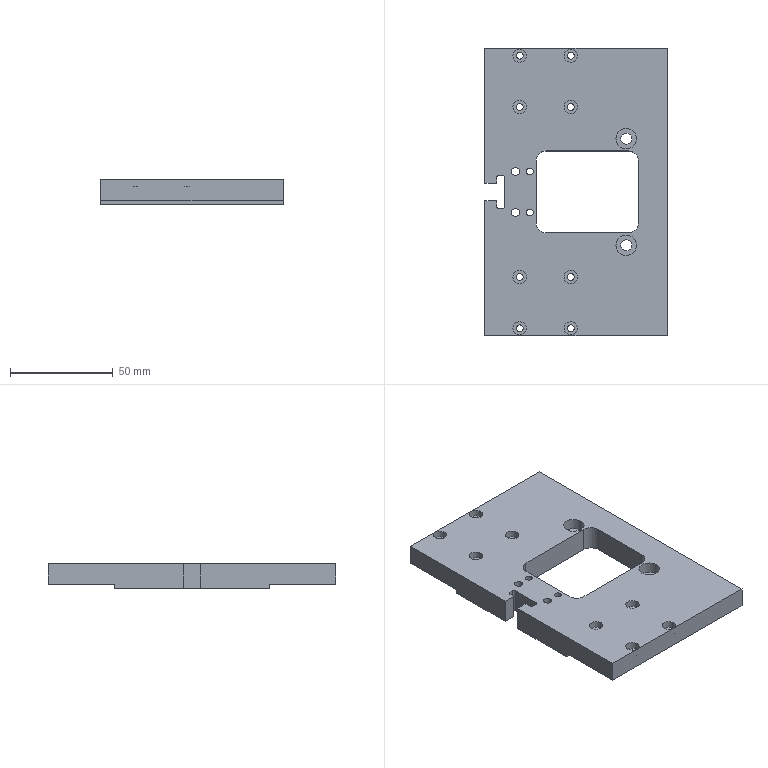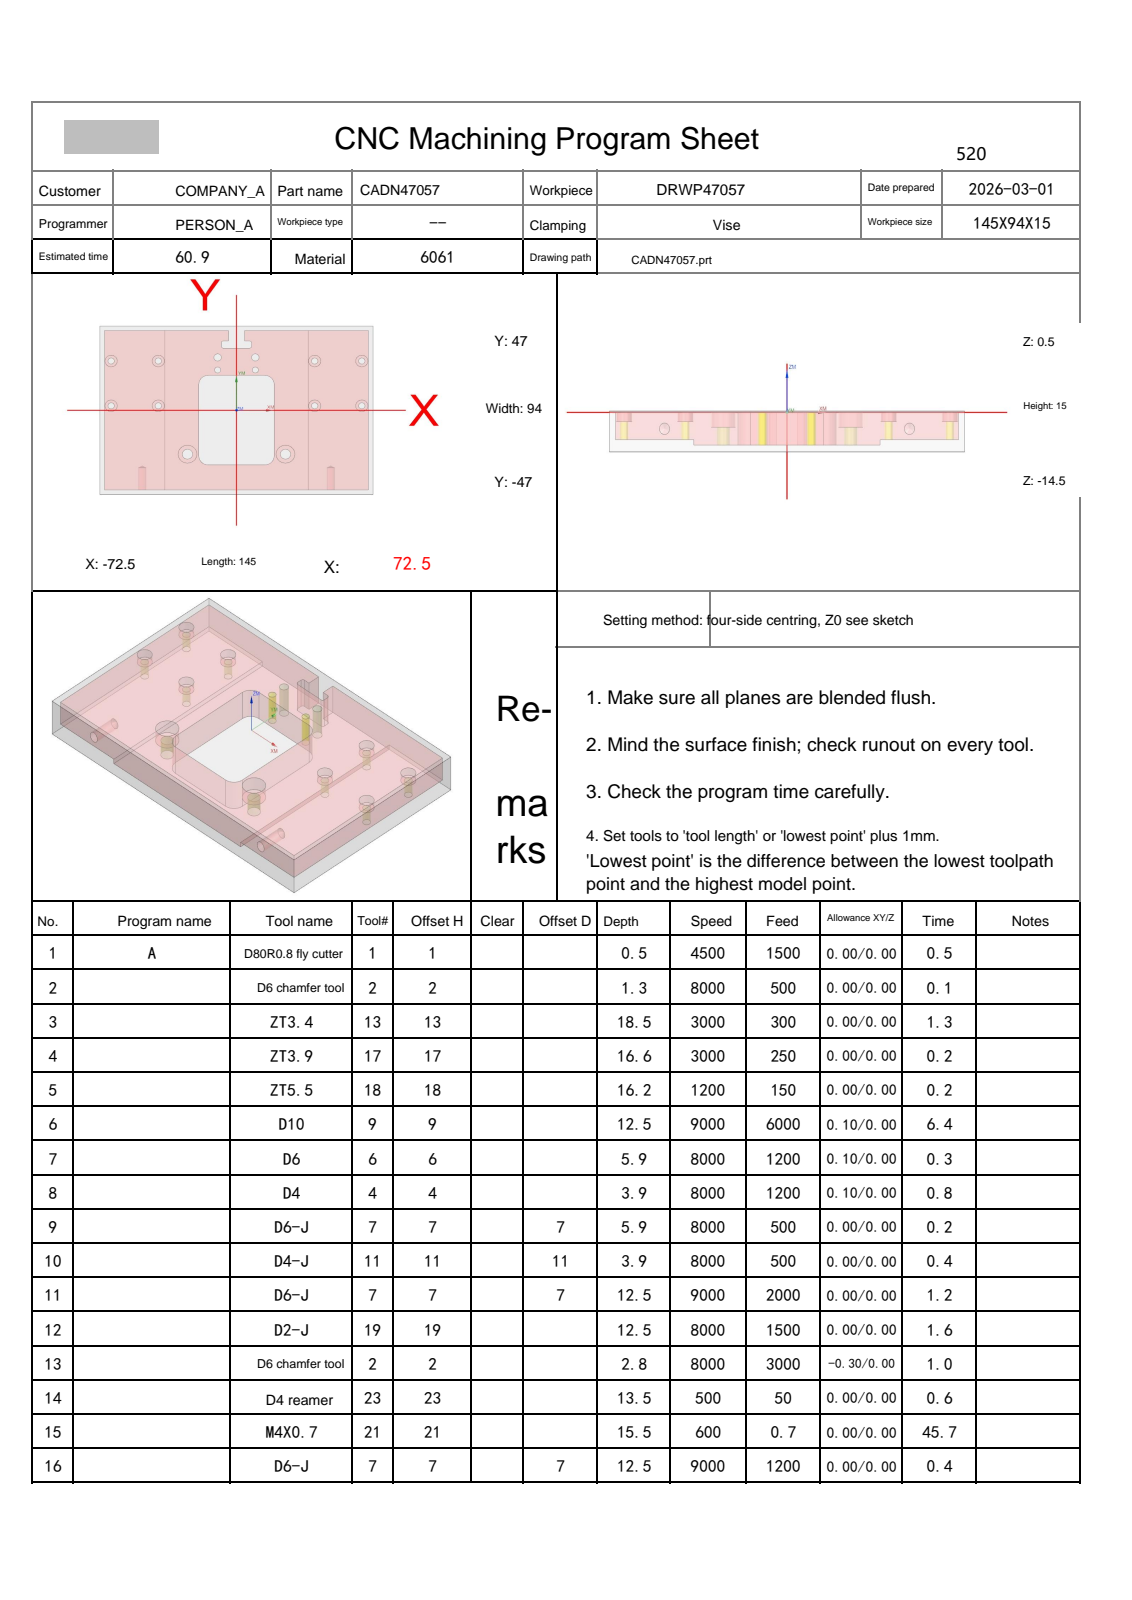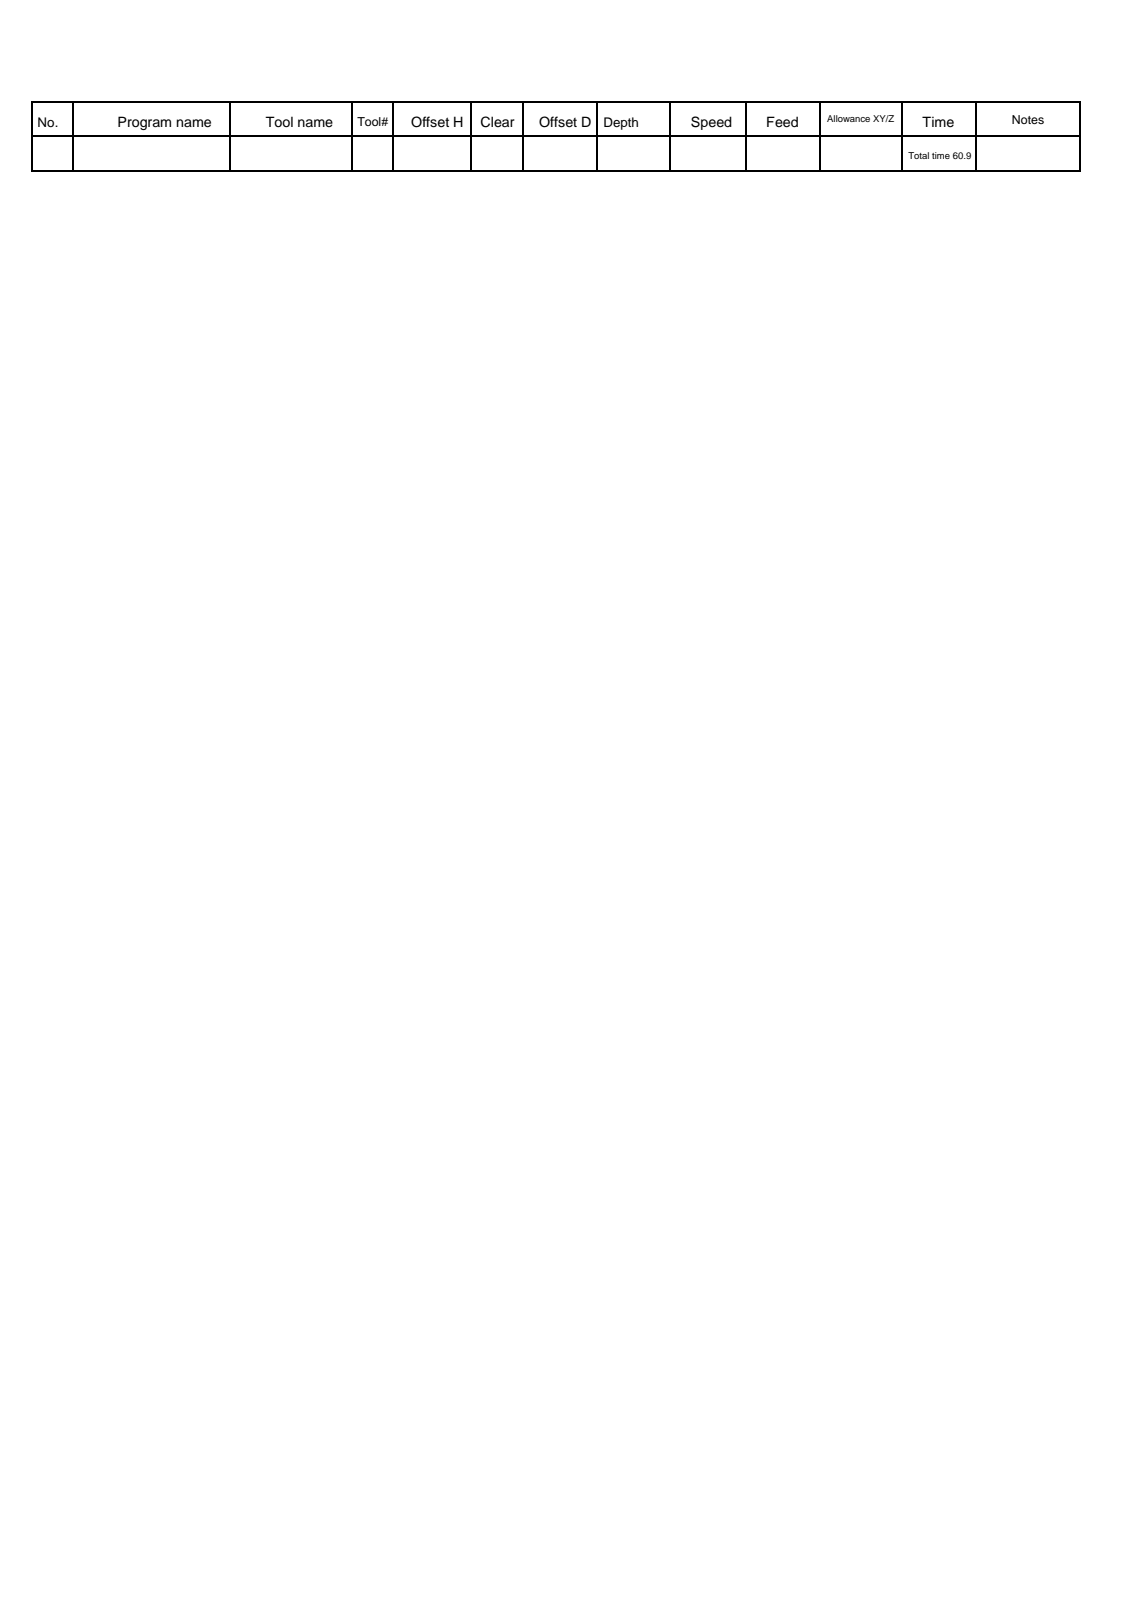NC program | NX | posted by the shop | part box 89 x 140 x 12 mm
Lines 1 to 948 of 6684:
%
O0001
(Machine time: 106.83 MIN)
(===Total Tool:13===)
(T1=D80R0.8 fly cutter D=80.  R=0.8  D-  H01 Z=0.    )
(T2=D6 chamfer tool   D=6.   R=0.   D-  H02 Z=-2.3  )
(T13=ZT3.4  D=3.4  DR_a=118 D-  H13 Z=-18.  )
(T17=ZT3.9  D=3.9  DR_a=120 D-  H17 Z=-16.13)
(T18=ZT5.5  D=5.5  DR_a=118 D-  H18 Z=-15.65)
(T9=D10     D=10.  R=0.   D-  H09 Z=-12.  )
(T6=D6      D=6.   R=0.   D-  H06 Z=-5.4  )
(T4=D4      D=4.   R=0.   D-  H04 Z=-3.4  )
(T7=D6-J    D=6.   R=0.   D7  H07 Z=-12.  )
(T11=D4-J   D=4.   R=0.   D11 H11 Z=-3.4  )
(T19=D2-J   D=2.   R=0.   D-  H19 Z=-12.  )
(T23=D4 reamer   D=4.   DR_a=180 D-  H23 Z=-13.  )
(T21=M4X0.7 D=3.3  DR_a=180 D-  H21 Z=-15.  )
G80 G90 G17 G49 G40
G91 G28 Z0
M01
N1 T01 M06
(D80R0.8 fly cutter  D=80. R=0.8 H=01 ce=0.00 di=0.00)
G00 G90 G54 X-115. Y42.25 M03 S4500
G43 H01 Z50.
M08
Z2.
G01 Z0.0 F1500.
X-110.
X110.
Y0.0
X-110.
Y-42.25
X110.
X115.
Z2.
G00 Z50.
G91 G28 Z0.0
M05
M09
G91 G28 Z0.0
M01
N2 T02 M06
(D6 chamfer tool  D=6. R=0. H=02 ce=0.00 di=0.00)
G00 G90 G54 X26. Y-24.5 M03 S8000
G43 H02 Z50.
M08
G98 G81 X26. Y-24.5 Z-.8 R1. F500.
X41.5 Y2.5
X66.5
Y27.5
X41.5
X10. Y29.5
Y22.5
X-10.
Y29.5
X-41.5 Y27.5
X-66.5
Y2.5
X-41.5
X-26. Y-24.5
G80
G00 Z50.
G91 G28 Z0.0
M05
M09
G91 G28 Z0.0
M01
N3 T13 M06
(ZT3.4 D=3.4 DR_a=118 H=13)
G00 G90 G54 X-10. Y22.5 M03 S3000
G43 H13 Z50.
M08
G98 G83 X-10. Y22.5 Z-18. R1. F300. Q2.
X10.
G80
G00 Z50.
G00 G90 X-66.5 Y2.5 M03 S2800
Z50.
G98 G83 X-66.5 Y2.5 Z-13.021 R1. F100. Q2.
Y27.5
X-41.5
Y2.5
X41.5
X66.5
Y27.5
X41.5
G80
G00 Z50.
G91 G28 Z0.0
M05
M09
G91 G28 Z0.0
M01
N4 T17 M06
(ZT3.9 D=3.9 DR_a=120 H=17)
G00 G90 G54 X-10. Y29.5 M03 S3000
G43 H17 Z50.
M08
G98 G83 X-10. Y29.5 Z-16.126 R1. F250. Q2.
X10.
G80
G00 Z50.
G91 G28 Z0.0
M05
M09
G91 G28 Z0.0
M01
N5 T18 M06
(ZT5.5 D=5.5 DR_a=118 H=18)
G00 G90 G54 X-26. Y-24.5 M03 S1200
G43 H18 Z50.
M08
G98 G83 X-26. Y-24.5 Z-15.652 R1. F150. Q2.
X26.
G80
G00 Z50.
G91 G28 Z0.0
M05
M09
G91 G28 Z0.0
M01
N6 T09 M06
(D10  D=10. R=0. H=09 ce=0.10 di=0.00)
G00 G90 G54 X14.9 Y-5.5 M03 S9000
G43 H09 Z50.
M08
Z.5
G01 Y14.4 Z.458 F1200.
X-14.9 Z.395
Y-25.4 Z.31
X14.9 Z.247
Y14.4 Z.163
X-14.9 Z.099
Y-25.4 Z.015
X14.9 Z-.048
Y14.4 Z-.133
X-14.9 Z-.196
Y-25.4 Z-.28
X14.9 Z-.344
Y14.4 Z-.428
X-14.9 Z-.491
Y-25.4 Z-.576
X14.9 Z-.639
Y14.4 Z-.723
X-14.9 Z-.786
Y-25.4 Z-.871
X14.9 Z-.934
Y14.4 Z-1.018
X-14.9 Z-1.082
Y-25.4 Z-1.166
X14.9 Z-1.229
Y14.4 Z-1.314
X-14.9 Z-1.377
Y-25.4 Z-1.461
X14.9 Z-1.524
Y14.4 Z-1.609
X-14.9 Z-1.672
Y-25.4 Z-1.756
X14.9 Z-1.82
Y14.4 Z-1.904
X-14.9 Z-1.967
Y-25.4 Z-2.052
X14.9 Z-2.115
Y14.4 Z-2.199
X-14.9 Z-2.263
Y-25.4 Z-2.347
X14.9 Z-2.41
Y14.4 Z-2.495
X-14.9 Z-2.558
Y-25.4 Z-2.642
X14.9 Z-2.705
Y14.4 Z-2.79
X-14.9 Z-2.853
Y-25.4 Z-2.937
X14.9 Z-3.001
Y14.4 Z-3.085
X-14.9 Z-3.148
Y-25.4 Z-3.233
X14.9 Z-3.296
Y14.4 Z-3.38
X-14.9 Z-3.444
Y-25.4 Z-3.528
X14.9 Z-3.591
Y14.4 Z-3.676
X-14.9 Z-3.739
Y-25.4 Z-3.823
X14.9 Z-3.886
Y14.4 Z-3.971
X-14.9 Z-4.034
Y-25.4 Z-4.118
X14.9 Z-4.182
Y14.4 Z-4.266
X-14.9 Z-4.329
Y-25.4 Z-4.414
X14.9 Z-4.477
Y14.4 Z-4.561
X-14.9 Z-4.624
Y-25.4 Z-4.709
X14.9 Z-4.772
Y14.4 Z-4.856
X-14.9 Z-4.92
Y-25.4 Z-5.004
X14.9 Z-5.067
Y14.4 Z-5.152
X-14.9 Z-5.215
Y-25.4 Z-5.299
X14.9 Z-5.363
Y14.4 Z-5.447
X-14.9 Z-5.51
Y-25.4 Z-5.595
X14.9 Z-5.658
Y14.4 Z-5.742
X-14.9 Z-5.805
Y-25.4 Z-5.89
X14.9 Z-5.953
Y14.4 Z-6.037
X-14.9 Z-6.101
Y-25.4 Z-6.185
X14.9 Z-6.248
Y14.4 Z-6.333
X-14.9 Z-6.396
Y-25.4 Z-6.48
X14.9 Z-6.544
Y14.4 Z-6.628
X-14.9 Z-6.691
Y-25.4 Z-6.776
X14.9 Z-6.839
Y14.4 Z-6.923
X-14.9 Z-6.986
Y-25.4 Z-7.071
X14.9 Z-7.134
Y14.4 Z-7.218
X-14.9 Z-7.282
Y-25.4 Z-7.366
X14.9 Z-7.429
Y14.4 Z-7.514
X-14.9 Z-7.577
Y-25.4 Z-7.661
X14.9 Z-7.724
Y14.4 Z-7.809
X-14.9 Z-7.872
Y-25.4 Z-7.956
X14.9 Z-8.02
Y14.4 Z-8.104
X-14.9 Z-8.167
Y-25.4 Z-8.252
X14.9 Z-8.315
Y14.4 Z-8.399
X-14.9 Z-8.463
Y-25.4 Z-8.547
X14.9 Z-8.61
Y14.4 Z-8.695
X-14.9 Z-8.758
Y-25.4 Z-8.842
X14.9 Z-8.905
Y14.4 Z-8.99
X-14.9 Z-9.053
Y-25.4 Z-9.137
X14.9 Z-9.201
Y14.4 Z-9.285
X-14.9 Z-9.348
Y-25.4 Z-9.433
X14.9 Z-9.496
Y14.4 Z-9.58
X-14.9 Z-9.644
Y-25.4 Z-9.728
X14.9 Z-9.791
Y14.4 Z-9.876
X-14.9 Z-9.939
Y-25.4 Z-10.023
X14.9 Z-10.086
Y14.4 Z-10.171
X-14.9 Z-10.234
Y-25.4 Z-10.318
X14.9 Z-10.382
Y14.4 Z-10.466
X-14.9 Z-10.529
Y-25.4 Z-10.614
X14.9 Z-10.677
Y14.4 Z-10.761
X-14.9 Z-10.824
Y-25.4 Z-10.909
X14.9 Z-10.972
Y14.4 Z-11.056
X-14.9 Z-11.12
Y-25.4 Z-11.204
X14.9 Z-11.267
Y14.4 Z-11.352
X-14.9 Z-11.415
Y-25.4 Z-11.499
X14.9 Z-11.563
Y14.4 Z-11.647
X-14.9 Z-11.71
Y-25.4 Z-11.795
X14.9 Z-11.858
Y-5.5 Z-11.9
Y14.4
X-14.9
Y-25.4
X14.9
Y-5.5
Y-5.
Z-10.9
G00 Z50.
G00 G90 X0.0 Y-49.6 M03 S8000
Z50.
Z.5
G01 X-70. Z.389 F6000.
G02 X-75.1 Y-44.5 Z.376 I0.0 J5.1
G01 Y44.5 Z.235
G02 X-70. Y49.6 Z.222 I5.1 J0.0
G01 X-4.25 Z.117
G02 X0.0 Y47.319 Z.109 I0.0 J-5.1
X4.25 Y49.6 Z.101 I4.25 J-2.819
G01 X70. Z-.003
G02 X75.1 Y44.5 Z-.016 I0.0 J-5.1
G01 Y-44.5 Z-.157
G02 X70. Y-49.6 Z-.17 I-5.1 J0.0
G01 X-70. Z-.392
G02 X-75.1 Y-44.5 Z-.405 I0.0 J5.1
G01 Y44.5 Z-.547
G02 X-70. Y49.6 Z-.559 I5.1 J0.0
G01 X-4.25 Z-.664
G02 X0.0 Y47.319 Z-.672 I0.0 J-5.1
X4.25 Y49.6 Z-.68 I4.25 J-2.819
G01 X70. Z-.784
G02 X75.1 Y44.5 Z-.797 I0.0 J-5.1
G01 Y-44.5 Z-.939
G02 X70. Y-49.6 Z-.951 I-5.1 J0.0
G01 X-70. Z-1.174
G02 X-75.1 Y-44.5 Z-1.186 I0.0 J5.1
G01 Y44.5 Z-1.328
G02 X-70. Y49.6 Z-1.341 I5.1 J0.0
G01 X-4.25 Z-1.445
G02 X0.0 Y47.319 Z-1.453 I0.0 J-5.1
X4.25 Y49.6 Z-1.461 I4.25 J-2.819
G01 X70. Z-1.566
G02 X75.1 Y44.5 Z-1.578 I0.0 J-5.1
G01 Y-44.5 Z-1.72
G02 X70. Y-49.6 Z-1.733 I-5.1 J0.0
G01 X-70. Z-1.955
G02 X-75.1 Y-44.5 Z-1.968 I0.0 J5.1
G01 Y44.5 Z-2.109
G02 X-70. Y49.6 Z-2.122 I5.1 J0.0
G01 X-4.25 Z-2.226
G02 X0.0 Y47.319 Z-2.234 I0.0 J-5.1
X4.25 Y49.6 Z-2.242 I4.25 J-2.819
G01 X70. Z-2.347
G02 X75.1 Y44.5 Z-2.36 I0.0 J-5.1
G01 Y-44.5 Z-2.501
G02 X70. Y-49.6 Z-2.514 I-5.1 J0.0
G01 X-70. Z-2.736
G02 X-75.1 Y-44.5 Z-2.749 I0.0 J5.1
G01 Y44.5 Z-2.89
G02 X-70. Y49.6 Z-2.903 I5.1 J0.0
G01 X-4.25 Z-3.008
G02 X0.0 Y47.319 Z-3.016 I0.0 J-5.1
X4.25 Y49.6 Z-3.024 I4.25 J-2.819
G01 X70. Z-3.128
G02 X75.1 Y44.5 Z-3.141 I0.0 J-5.1
G01 Y-44.5 Z-3.282
G02 X70. Y-49.6 Z-3.295 I-5.1 J0.0
G01 X-70. Z-3.517
G02 X-75.1 Y-44.5 Z-3.53 I0.0 J5.1
G01 Y44.5 Z-3.672
G02 X-70. Y49.6 Z-3.684 I5.1 J0.0
G01 X-4.25 Z-3.789
G02 X0.0 Y47.319 Z-3.797 I0.0 J-5.1
X4.25 Y49.6 Z-3.805 I4.25 J-2.819
G01 X70. Z-3.909
G02 X75.1 Y44.5 Z-3.922 I0.0 J-5.1
G01 Y-44.5 Z-4.064
G02 X70. Y-49.6 Z-4.076 I-5.1 J0.0
G01 X-70. Z-4.299
G02 X-75.1 Y-44.5 Z-4.311 I0.0 J5.1
G01 Y44.5 Z-4.453
G02 X-70. Y49.6 Z-4.466 I5.1 J0.0
G01 X-4.25 Z-4.57
G02 X0.0 Y47.319 Z-4.578 I0.0 J-5.1
X4.25 Y49.6 Z-4.586 I4.25 J-2.819
G01 X70. Z-4.691
G02 X75.1 Y44.5 Z-4.703 I0.0 J-5.1
G01 Y-44.5 Z-4.845
G02 X70. Y-49.6 Z-4.858 I-5.1 J0.0
G01 X-70. Z-5.08
G02 X-75.1 Y-44.5 Z-5.093 I0.0 J5.1
G01 Y44.5 Z-5.234
G02 X-70. Y49.6 Z-5.247 I5.1 J0.0
G01 X-4.25 Z-5.351
G02 X0.0 Y47.319 Z-5.359 I0.0 J-5.1
X4.25 Y49.6 Z-5.367 I4.25 J-2.819
G01 X70. Z-5.472
G02 X75.1 Y44.5 Z-5.485 I0.0 J-5.1
G01 Y-44.5 Z-5.626
G02 X70. Y-49.6 Z-5.639 I-5.1 J0.0
G01 X-70. Z-5.861
G02 X-75.1 Y-44.5 Z-5.874 I0.0 J5.1
G01 Y44.5 Z-6.015
G02 X-70. Y49.6 Z-6.028 I5.1 J0.0
G01 X-4.25 Z-6.133
G02 X0.0 Y47.319 Z-6.141 I0.0 J-5.1
X4.25 Y49.6 Z-6.149 I4.25 J-2.819
G01 X70. Z-6.253
G02 X75.1 Y44.5 Z-6.266 I0.0 J-5.1
G01 Y-44.5 Z-6.407
G02 X70. Y-49.6 Z-6.42 I-5.1 J0.0
G01 X-70. Z-6.642
G02 X-75.1 Y-44.5 Z-6.655 I0.0 J5.1
G01 Y44.5 Z-6.797
G02 X-70. Y49.6 Z-6.809 I5.1 J0.0
G01 X-4.25 Z-6.914
G02 X0.0 Y47.319 Z-6.922 I0.0 J-5.1
X4.25 Y49.6 Z-6.93 I4.25 J-2.819
G01 X70. Z-7.034
G02 X75.1 Y44.5 Z-7.047 I0.0 J-5.1
G01 Y-44.5 Z-7.189
G02 X70. Y-49.6 Z-7.201 I-5.1 J0.0
G01 X-70. Z-7.424
G02 X-75.1 Y-44.5 Z-7.436 I0.0 J5.1
G01 Y44.5 Z-7.578
G02 X-70. Y49.6 Z-7.591 I5.1 J0.0
G01 X-4.25 Z-7.695
G02 X0.0 Y47.319 Z-7.703 I0.0 J-5.1
X4.25 Y49.6 Z-7.711 I4.25 J-2.819
G01 X70. Z-7.816
G02 X75.1 Y44.5 Z-7.828 I0.0 J-5.1
G01 Y-44.5 Z-7.97
G02 X70. Y-49.6 Z-7.983 I-5.1 J0.0
G01 X-70. Z-8.205
G02 X-75.1 Y-44.5 Z-8.218 I0.0 J5.1
G01 Y44.5 Z-8.359
G02 X-70. Y49.6 Z-8.372 I5.1 J0.0
G01 X-4.25 Z-8.476
G02 X0.0 Y47.319 Z-8.484 I0.0 J-5.1
X4.25 Y49.6 Z-8.492 I4.25 J-2.819
G01 X70. Z-8.597
G02 X75.1 Y44.5 Z-8.61 I0.0 J-5.1
G01 Y-44.5 Z-8.751
G02 X70. Y-49.6 Z-8.764 I-5.1 J0.0
G01 X-70. Z-8.986
G02 X-75.1 Y-44.5 Z-8.999 I0.0 J5.1
G01 Y44.5 Z-9.14
G02 X-70. Y49.6 Z-9.153 I5.1 J0.0
G01 X-4.25 Z-9.258
G02 X0.0 Y47.319 Z-9.266 I0.0 J-5.1
X4.25 Y49.6 Z-9.274 I4.25 J-2.819
G01 X70. Z-9.378
G02 X75.1 Y44.5 Z-9.391 I0.0 J-5.1
G01 Y-44.5 Z-9.532
G02 X70. Y-49.6 Z-9.545 I-5.1 J0.0
G01 X-70. Z-9.767
G02 X-75.1 Y-44.5 Z-9.78 I0.0 J5.1
G01 Y44.5 Z-9.922
G02 X-70. Y49.6 Z-9.934 I5.1 J0.0
G01 X-4.25 Z-10.039
G02 X0.0 Y47.319 Z-10.047 I0.0 J-5.1
X4.25 Y49.6 Z-10.055 I4.25 J-2.819
G01 X70. Z-10.159
G02 X75.1 Y44.5 Z-10.172 I0.0 J-5.1
G01 Y-44.5 Z-10.314
G02 X70. Y-49.6 Z-10.326 I-5.1 J0.0
G01 X-70. Z-10.549
G02 X-75.1 Y-44.5 Z-10.561 I0.0 J5.1
G01 Y44.5 Z-10.703
G02 X-70. Y49.6 Z-10.716 I5.1 J0.0
G01 X-4.25 Z-10.82
G02 X0.0 Y47.319 Z-10.828 I0.0 J-5.1
X4.25 Y49.6 Z-10.836 I4.25 J-2.819
G01 X70. Z-10.941
G02 X75.1 Y44.5 Z-10.953 I0.0 J-5.1
G01 Y-44.5 Z-11.095
G02 X70. Y-49.6 Z-11.108 I-5.1 J0.0
G01 X-70. Z-11.33
G02 X-75.1 Y-44.5 Z-11.343 I0.0 J5.1
G01 Y44.5 Z-11.484
G02 X-70. Y49.6 Z-11.497 I5.1 J0.0
G01 X-4.25 Z-11.601
G02 X0.0 Y47.319 Z-11.609 I0.0 J-5.1
X4.25 Y49.6 Z-11.617 I4.25 J-2.819
G01 X70. Z-11.722
G02 X75.1 Y44.5 Z-11.735 I0.0 J-5.1
G01 Y-44.5 Z-11.876
G02 X70. Y-49.6 Z-11.889 I-5.1 J0.0
G01 X0.0 Z-12.
X-70.
G02 X-75.1 Y-44.5 I0.0 J5.1
G01 Y44.5
G02 X-70. Y49.6 I5.1 J0.0
G01 X-4.25
G02 X0.0 Y47.319 I0.0 J-5.1
X4.25 Y49.6 I4.25 J-2.819
G01 X70.
G02 X75.1 Y44.5 I0.0 J-5.1
G01 Y-44.5
G02 X70. Y-49.6 I-5.1 J0.0
G01 X0.0
X-.5
Z-11.
G00 Z50.
G91 G28 Z0.0
M05
M09
G91 G28 Z0.0
M01
N7 T06 M06
(D6  D=6. R=0. H=06 ce=0.10 di=0.00)
G00 G90 G54 X-26. Y-24.5 M03 S8000
G43 H06 Z50.
M08
Z.5
G03 X-26.95 Y-25.45 I0.0 J-.95 F1200.
X-26. Y-26.4 I.95 J0.0
X-26. Y-26.4 Z0.0 I0.0 J1.9
X-26. Y-26.4 Z-.5 I0.0 J1.9
X-26. Y-26.4 Z-1. I0.0 J1.9
X-26. Y-26.4 Z-1.5 I0.0 J1.9
X-26. Y-26.4 Z-2. I0.0 J1.9
X-26. Y-26.4 Z-2.5 I0.0 J1.9
X-26. Y-26.4 Z-3. I0.0 J1.9
X-26. Y-26.4 Z-3.5 I0.0 J1.9
X-26. Y-26.4 Z-4. I0.0 J1.9
X-26. Y-26.4 Z-4.5 I0.0 J1.9
X-26. Y-26.4 Z-5. I0.0 J1.9
X-27.807 Y-25.087 Z-5.4 I0.0 J1.9
X-26. Y-26.4 I1.807 J.587
X-24.1 Y-24.5 I0.0 J1.9
X-26. Y-22.6 I-1.9 J0.0
X-27.9 Y-24.5 I0.0 J-1.9
X-27.807 Y-25.087 I1.9 J0.0
X-26.904 Y-25.744 I.904 J.294
X-25.954 Y-24.794 I0.0 J.95
X-26. Y-24.5 I-.95 J0.0
G00 Z50.
X26.
Z.5
G03 X25.05 Y-25.45 I0.0 J-.95
X26. Y-26.4 I.95 J0.0
X26. Y-26.4 Z0.0 I0.0 J1.9
X26. Y-26.4 Z-.5 I0.0 J1.9
X26. Y-26.4 Z-1. I0.0 J1.9
X26. Y-26.4 Z-1.5 I0.0 J1.9
X26. Y-26.4 Z-2. I0.0 J1.9
X26. Y-26.4 Z-2.5 I0.0 J1.9
X26. Y-26.4 Z-3. I0.0 J1.9
X26. Y-26.4 Z-3.5 I0.0 J1.9
X26. Y-26.4 Z-4. I0.0 J1.9
X26. Y-26.4 Z-4.5 I0.0 J1.9
X26. Y-26.4 Z-5. I0.0 J1.9
X24.193 Y-25.087 Z-5.4 I0.0 J1.9
X26. Y-26.4 I1.807 J.587
X27.9 Y-24.5 I0.0 J1.9
X26. Y-22.6 I-1.9 J0.0
X24.1 Y-24.5 I0.0 J-1.9
X24.193 Y-25.087 I1.9 J0.0
X25.096 Y-25.744 I.904 J.294
X26.046 Y-24.794 I0.0 J.95
X26. Y-24.5 I-.95 J0.0
G00 Z50.
G91 G28 Z0.0
M05
M09
G91 G28 Z0.0
M01
N8 T04 M06
(D4  D=4. R=0. H=04 ce=0.10 di=0.00)
G00 G90 G54 X-66.5 Y2.5 M03 S8000
G43 H04 Z50.
M08
Z.5
G03 X-67.075 Y1.925 I0.0 J-.575 F1200.
X-66.5 Y1.35 I.575 J0.0
X-66.5 Y1.35 Z.2 I0.0 J1.15
X-66.5 Y1.35 Z-.1 I0.0 J1.15
X-66.5 Y1.35 Z-.4 I0.0 J1.15
X-66.5 Y1.35 Z-.7 I0.0 J1.15
X-66.5 Y1.35 Z-1. I0.0 J1.15
X-66.5 Y1.35 Z-1.3 I0.0 J1.15
X-66.5 Y1.35 Z-1.6 I0.0 J1.15
X-66.5 Y1.35 Z-1.9 I0.0 J1.15
X-66.5 Y1.35 Z-2.2 I0.0 J1.15
X-66.5 Y1.35 Z-2.5 I0.0 J1.15
X-66.5 Y1.35 Z-2.8 I0.0 J1.15
X-66.5 Y1.35 Z-3.1 I0.0 J1.15
X-66.5 Y1.35 Z-3.4 I0.0 J1.15
X-65.35 Y2.5 I0.0 J1.15
X-66.5 Y3.65 I-1.15 J0.0
X-67.65 Y2.5 I0.0 J-1.15
X-66.5 Y1.35 I1.15 J0.0
X-65.925 Y1.925 I0.0 J.575
X-66.5 Y2.5 I-.575 J0.0
G00 Z50.
Y27.5
Z.5
G03 X-67.075 Y26.925 I0.0 J-.575
X-66.5 Y26.35 I.575 J0.0
X-66.5 Y26.35 Z.2 I0.0 J1.15
X-66.5 Y26.35 Z-.1 I0.0 J1.15
X-66.5 Y26.35 Z-.4 I0.0 J1.15
X-66.5 Y26.35 Z-.7 I0.0 J1.15
X-66.5 Y26.35 Z-1. I0.0 J1.15
X-66.5 Y26.35 Z-1.3 I0.0 J1.15
X-66.5 Y26.35 Z-1.6 I0.0 J1.15
X-66.5 Y26.35 Z-1.9 I0.0 J1.15
X-66.5 Y26.35 Z-2.2 I0.0 J1.15
X-66.5 Y26.35 Z-2.5 I0.0 J1.15
X-66.5 Y26.35 Z-2.8 I0.0 J1.15
X-66.5 Y26.35 Z-3.1 I0.0 J1.15
X-66.5 Y26.35 Z-3.4 I0.0 J1.15
X-65.35 Y27.5 I0.0 J1.15
X-66.5 Y28.65 I-1.15 J0.0
X-67.65 Y27.5 I0.0 J-1.15
X-66.5 Y26.35 I1.15 J0.0
X-65.925 Y26.925 I0.0 J.575
X-66.5 Y27.5 I-.575 J0.0
G00 Z50.
X-41.5
Z.5
G03 X-42.075 Y26.925 I0.0 J-.575
X-41.5 Y26.35 I.575 J0.0
X-41.5 Y26.35 Z.2 I0.0 J1.15
X-41.5 Y26.35 Z-.1 I0.0 J1.15
X-41.5 Y26.35 Z-.4 I0.0 J1.15
X-41.5 Y26.35 Z-.7 I0.0 J1.15
X-41.5 Y26.35 Z-1. I0.0 J1.15
X-41.5 Y26.35 Z-1.3 I0.0 J1.15
X-41.5 Y26.35 Z-1.6 I0.0 J1.15
X-41.5 Y26.35 Z-1.9 I0.0 J1.15
X-41.5 Y26.35 Z-2.2 I0.0 J1.15
X-41.5 Y26.35 Z-2.5 I0.0 J1.15
X-41.5 Y26.35 Z-2.8 I0.0 J1.15
X-41.5 Y26.35 Z-3.1 I0.0 J1.15
X-41.5 Y26.35 Z-3.4 I0.0 J1.15
X-40.35 Y27.5 I0.0 J1.15
X-41.5 Y28.65 I-1.15 J0.0
X-42.65 Y27.5 I0.0 J-1.15
X-41.5 Y26.35 I1.15 J0.0
X-40.925 Y26.925 I0.0 J.575
X-41.5 Y27.5 I-.575 J0.0
G00 Z50.
Y2.5
Z.5
G03 X-42.075 Y1.925 I0.0 J-.575
X-41.5 Y1.35 I.575 J0.0
X-41.5 Y1.35 Z.2 I0.0 J1.15
X-41.5 Y1.35 Z-.1 I0.0 J1.15
X-41.5 Y1.35 Z-.4 I0.0 J1.15
X-41.5 Y1.35 Z-.7 I0.0 J1.15
X-41.5 Y1.35 Z-1. I0.0 J1.15
X-41.5 Y1.35 Z-1.3 I0.0 J1.15
X-41.5 Y1.35 Z-1.6 I0.0 J1.15
X-41.5 Y1.35 Z-1.9 I0.0 J1.15
X-41.5 Y1.35 Z-2.2 I0.0 J1.15
X-41.5 Y1.35 Z-2.5 I0.0 J1.15
X-41.5 Y1.35 Z-2.8 I0.0 J1.15
X-41.5 Y1.35 Z-3.1 I0.0 J1.15
X-41.5 Y1.35 Z-3.4 I0.0 J1.15
X-40.35 Y2.5 I0.0 J1.15
X-41.5 Y3.65 I-1.15 J0.0
X-42.65 Y2.5 I0.0 J-1.15
X-41.5 Y1.35 I1.15 J0.0
X-40.925 Y1.925 I0.0 J.575
X-41.5 Y2.5 I-.575 J0.0
G00 Z50.
X41.5
Z.5
G03 X40.925 Y1.925 I0.0 J-.575
X41.5 Y1.35 I.575 J0.0
X41.5 Y1.35 Z.2 I0.0 J1.15
X41.5 Y1.35 Z-.1 I0.0 J1.15
X41.5 Y1.35 Z-.4 I0.0 J1.15
X41.5 Y1.35 Z-.7 I0.0 J1.15
X41.5 Y1.35 Z-1. I0.0 J1.15
X41.5 Y1.35 Z-1.3 I0.0 J1.15
X41.5 Y1.35 Z-1.6 I0.0 J1.15
X41.5 Y1.35 Z-1.9 I0.0 J1.15
X41.5 Y1.35 Z-2.2 I0.0 J1.15
X41.5 Y1.35 Z-2.5 I0.0 J1.15
X41.5 Y1.35 Z-2.8 I0.0 J1.15
X41.5 Y1.35 Z-3.1 I0.0 J1.15
X41.5 Y1.35 Z-3.4 I0.0 J1.15
X42.65 Y2.5 I0.0 J1.15
X41.5 Y3.65 I-1.15 J0.0
X40.35 Y2.5 I0.0 J-1.15
X41.5 Y1.35 I1.15 J0.0
X42.075 Y1.925 I0.0 J.575
X41.5 Y2.5 I-.575 J0.0
G00 Z50.
X66.5
Z.5
G03 X65.925 Y1.925 I0.0 J-.575
X66.5 Y1.35 I.575 J0.0
X66.5 Y1.35 Z.2 I0.0 J1.15
X66.5 Y1.35 Z-.1 I0.0 J1.15
X66.5 Y1.35 Z-.4 I0.0 J1.15
X66.5 Y1.35 Z-.7 I0.0 J1.15
X66.5 Y1.35 Z-1. I0.0 J1.15
X66.5 Y1.35 Z-1.3 I0.0 J1.15
X66.5 Y1.35 Z-1.6 I0.0 J1.15
X66.5 Y1.35 Z-1.9 I0.0 J1.15
X66.5 Y1.35 Z-2.2 I0.0 J1.15
X66.5 Y1.35 Z-2.5 I0.0 J1.15
X66.5 Y1.35 Z-2.8 I0.0 J1.15
X66.5 Y1.35 Z-3.1 I0.0 J1.15
X66.5 Y1.35 Z-3.4 I0.0 J1.15
X67.65 Y2.5 I0.0 J1.15
X66.5 Y3.65 I-1.15 J0.0
X65.35 Y2.5 I0.0 J-1.15
X66.5 Y1.35 I1.15 J0.0
X67.075 Y1.925 I0.0 J.575
X66.5 Y2.5 I-.575 J0.0
G00 Z50.
Y27.5
Z.5
G03 X65.925 Y26.925 I0.0 J-.575
X66.5 Y26.35 I.575 J0.0
X66.5 Y26.35 Z.2 I0.0 J1.15
X66.5 Y26.35 Z-.1 I0.0 J1.15
X66.5 Y26.35 Z-.4 I0.0 J1.15
X66.5 Y26.35 Z-.7 I0.0 J1.15
X66.5 Y26.35 Z-1. I0.0 J1.15
X66.5 Y26.35 Z-1.3 I0.0 J1.15
X66.5 Y26.35 Z-1.6 I0.0 J1.15
X66.5 Y26.35 Z-1.9 I0.0 J1.15
X66.5 Y26.35 Z-2.2 I0.0 J1.15
X66.5 Y26.35 Z-2.5 I0.0 J1.15
X66.5 Y26.35 Z-2.8 I0.0 J1.15
X66.5 Y26.35 Z-3.1 I0.0 J1.15
X66.5 Y26.35 Z-3.4 I0.0 J1.15
X67.65 Y27.5 I0.0 J1.15
X66.5 Y28.65 I-1.15 J0.0
X65.35 Y27.5 I0.0 J-1.15
X66.5 Y26.35 I1.15 J0.0
X67.075 Y26.925 I0.0 J.575
X66.5 Y27.5 I-.575 J0.0
G00 Z50.
X41.5
Z.5
G03 X40.925 Y26.925 I0.0 J-.575
X41.5 Y26.35 I.575 J0.0
X41.5 Y26.35 Z.2 I0.0 J1.15
X41.5 Y26.35 Z-.1 I0.0 J1.15
X41.5 Y26.35 Z-.4 I0.0 J1.15
X41.5 Y26.35 Z-.7 I0.0 J1.15
X41.5 Y26.35 Z-1. I0.0 J1.15
X41.5 Y26.35 Z-1.3 I0.0 J1.15
X41.5 Y26.35 Z-1.6 I0.0 J1.15
X41.5 Y26.35 Z-1.9 I0.0 J1.15
X41.5 Y26.35 Z-2.2 I0.0 J1.15
X41.5 Y26.35 Z-2.5 I0.0 J1.15
X41.5 Y26.35 Z-2.8 I0.0 J1.15
X41.5 Y26.35 Z-3.1 I0.0 J1.15
X41.5 Y26.35 Z-3.4 I0.0 J1.15
X42.65 Y27.5 I0.0 J1.15
X41.5 Y28.65 I-1.15 J0.0
X40.35 Y27.5 I0.0 J-1.15
X41.5 Y26.35 I1.15 J0.0
X42.075 Y26.925 I0.0 J.575
X41.5 Y27.5 I-.575 J0.0
G00 Z50.
G91 G28 Z0.0
M05
M09
G91 G28 Z0.0
M01
N9 T07 M06
(D6-J  D=6. R=0. H=07 ce=0.00 di=0.00)
G00 G90 G54 X-26. Y-24.5 M03 S8000
G43 H07 Z50.
M08
Z0.0
G41 D07
G01 X-26.196 Y-24.54 F500.
G03 X-26.99 Y-25.51 I.196 J-.97
X-26. Y-26.5 I.99 J0.0
X-26. Y-26.5 Z-5. I0.0 J2.
X-25.036 Y-26.253 Z-5.4 I0.0 J2.
X-24. Y-24.5 I-.964 J1.753
X-26. Y-22.5 I-2. J0.0
X-28. Y-24.5 I0.0 J-2.
X-26. Y-26.5 I2. J0.0
X-25.036 Y-26.253 I0.0 J2.
X-24.523 Y-25.385 I-.477 J.868
X-25.513 Y-24.395 I-.99 J0.0
X-25.809 Y-24.44 I0.0 J-.99
G01 G40 X-26. Y-24.5
G00 Z50.
X26.
Z0.0
G41 D07
G01 X25.804 Y-24.54
G03 X25.01 Y-25.51 I.196 J-.97
X26. Y-26.5 I.99 J0.0
X26. Y-26.5 Z-5. I0.0 J2.
X26.964 Y-26.253 Z-5.4 I0.0 J2.
X28. Y-24.5 I-.964 J1.753
X26. Y-22.5 I-2. J0.0
X24. Y-24.5 I0.0 J-2.
X26. Y-26.5 I2. J0.0
X26.964 Y-26.253 I0.0 J2.
X27.477 Y-25.385 I-.477 J.868
X26.487 Y-24.395 I-.99 J0.0
X26.191 Y-24.44 I0.0 J-.99
G01 G40 X26. Y-24.5
G00 Z50.
G91 G28 Z0.0
M05
M09
G91 G28 Z0.0
M01
N10 T11 M06
(D4-J  D=4. R=0. H=11 ce=0.00 di=0.00)
G00 G90 G54 X-66.5 Y2.5 M03 S8000
G43 H11 Z50.
M08
Z.5
G41 D11
G01 X-66.69 Y2.438 F500.
G03 X-67.109 Y1.859 I.19 J-.579
X-66.5 Y1.25 I.609 J0.0
X-67.728 Y2.266 Z-3.4 I0.0 J1.25
X-66.5 Y1.25 I1.228 J.234
X-65.25 Y2.5 I0.0 J1.25
X-66.5 Y3.75 I-1.25 J0.0
X-67.75 Y2.5 I0.0 J-1.25
X-67.728 Y2.266 I1.25 J0.0
X-67.13 Y1.771 I.598 J.114
X-66.526 Y2.302 I0.0 J.609
G01 G40 X-66.5 Y2.5
G00 Z50.
Y27.5
Z.5
G41 D11
G01 X-66.69 Y27.438
G03 X-67.109 Y26.859 I.19 J-.579
X-66.5 Y26.25 I.609 J0.0
X-67.728 Y27.266 Z-3.4 I0.0 J1.25
X-66.5 Y26.25 I1.228 J.234
X-65.25 Y27.5 I0.0 J1.25
X-66.5 Y28.75 I-1.25 J0.0
X-67.75 Y27.5 I0.0 J-1.25
X-67.728 Y27.266 I1.25 J0.0
X-67.13 Y26.771 I.598 J.114
X-66.526 Y27.302 I0.0 J.609
G01 G40 X-66.5 Y27.5
G00 Z50.
X-41.5
Z.5
G41 D11
G01 X-41.69 Y27.438
G03 X-42.109 Y26.859 I.19 J-.579
X-41.5 Y26.25 I.609 J0.0
X-42.728 Y27.266 Z-3.4 I0.0 J1.25
X-41.5 Y26.25 I1.228 J.234
X-40.25 Y27.5 I0.0 J1.25
X-41.5 Y28.75 I-1.25 J0.0
X-42.75 Y27.5 I0.0 J-1.25
X-42.728 Y27.266 I1.25 J0.0
X-42.13 Y26.771 I.598 J.114
X-41.526 Y27.302 I0.0 J.609
G01 G40 X-41.5 Y27.5
G00 Z50.
Y2.5
Z.5
G41 D11
G01 X-41.69 Y2.438
G03 X-42.109 Y1.859 I.19 J-.579
X-41.5 Y1.25 I.609 J0.0
X-42.728 Y2.266 Z-3.4 I0.0 J1.25
X-41.5 Y1.25 I1.228 J.234
X-40.25 Y2.5 I0.0 J1.25
X-41.5 Y3.75 I-1.25 J0.0
X-42.75 Y2.5 I0.0 J-1.25
X-42.728 Y2.266 I1.25 J0.0
X-42.13 Y1.771 I.598 J.114
X-41.526 Y2.302 I0.0 J.609
G01 G40 X-41.5 Y2.5
G00 Z50.
X41.5
Z.5
G41 D11
G01 X41.31 Y2.438
G03 X40.891 Y1.859 I.19 J-.579
X41.5 Y1.25 I.609 J0.0
X40.272 Y2.266 Z-3.4 I0.0 J1.25
X41.5 Y1.25 I1.228 J.234
X42.75 Y2.5 I0.0 J1.25
X41.5 Y3.75 I-1.25 J0.0
X40.25 Y2.5 I0.0 J-1.25
X40.272 Y2.266 I1.25 J0.0
X40.87 Y1.771 I.598 J.114
X41.474 Y2.302 I0.0 J.609
G01 G40 X41.5 Y2.5
G00 Z50.
X66.5
Z.5
G41 D11
G01 X66.31 Y2.438
G03 X65.891 Y1.859 I.19 J-.579
X66.5 Y1.25 I.609 J0.0
X65.272 Y2.266 Z-3.4 I0.0 J1.25
X66.5 Y1.25 I1.228 J.234
X67.75 Y2.5 I0.0 J1.25
X66.5 Y3.75 I-1.25 J0.0
X65.25 Y2.5 I0.0 J-1.25
X65.272 Y2.266 I1.25 J0.0
X65.87 Y1.771 I.598 J.114
X66.474 Y2.302 I0.0 J.609
G01 G40 X66.5 Y2.5
G00 Z50.
Y27.5
Z.5
G41 D11
G01 X66.31 Y27.438
G03 X65.891 Y26.859 I.19 J-.579
X66.5 Y26.25 I.609 J0.0
X65.272 Y27.266 Z-3.4 I0.0 J1.25
X66.5 Y26.25 I1.228 J.234
X67.75 Y27.5 I0.0 J1.25
X66.5 Y28.75 I-1.25 J0.0
X65.25 Y27.5 I0.0 J-1.25
X65.272 Y27.266 I1.25 J0.0
X65.87 Y26.771 I.598 J.114
X66.474 Y27.302 I0.0 J.609
G01 G40 X66.5 Y27.5
G00 Z50.
X41.5
Z.5
G41 D11
G01 X41.31 Y27.438
G03 X40.891 Y26.859 I.19 J-.579
X41.5 Y26.25 I.609 J0.0
X40.272 Y27.266 Z-3.4 I0.0 J1.25
X41.5 Y26.25 I1.228 J.234
X42.75 Y27.5 I0.0 J1.25
X41.5 Y28.75 I-1.25 J0.0
X40.25 Y27.5 I0.0 J-1.25
X40.272 Y27.266 I1.25 J0.0
X40.87 Y26.771 I.598 J.114
X41.474 Y27.302 I0.0 J.609
G01 G40 X41.5 Y27.5
G00 Z50.
G91 G28 Z0.0
M05
M09
G91 G28 Z0.0
M01